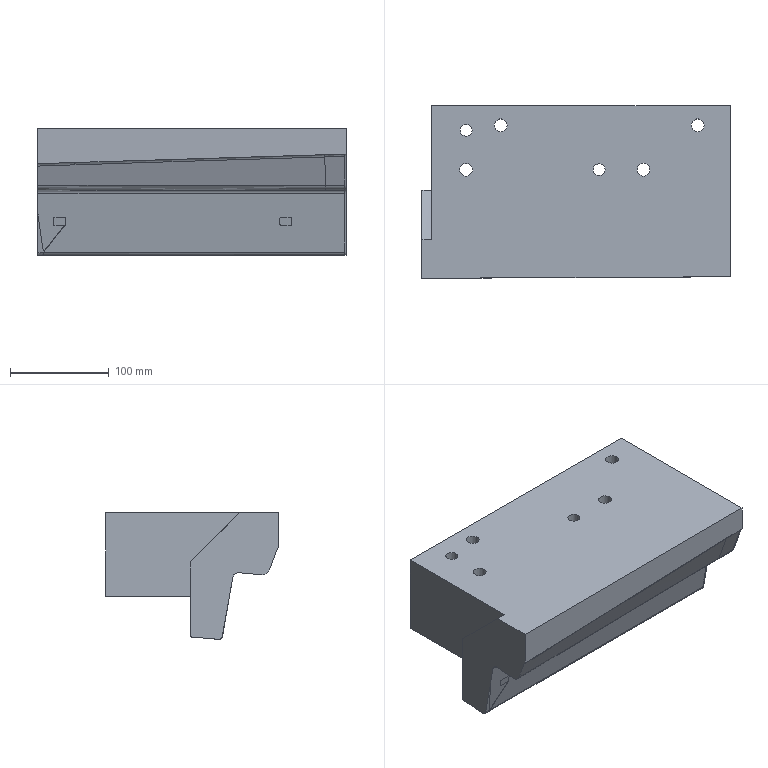Part | NX | features solid 2 | 1 solid | 54 faces | box 312.901 x 175.24 x 128.578 mm | volume 4371113 mm3 | spline 29 | plane 13 | cylinder 12 | commonest cylinder face diameters 13 x4 20 x4 12 x2 16 x2